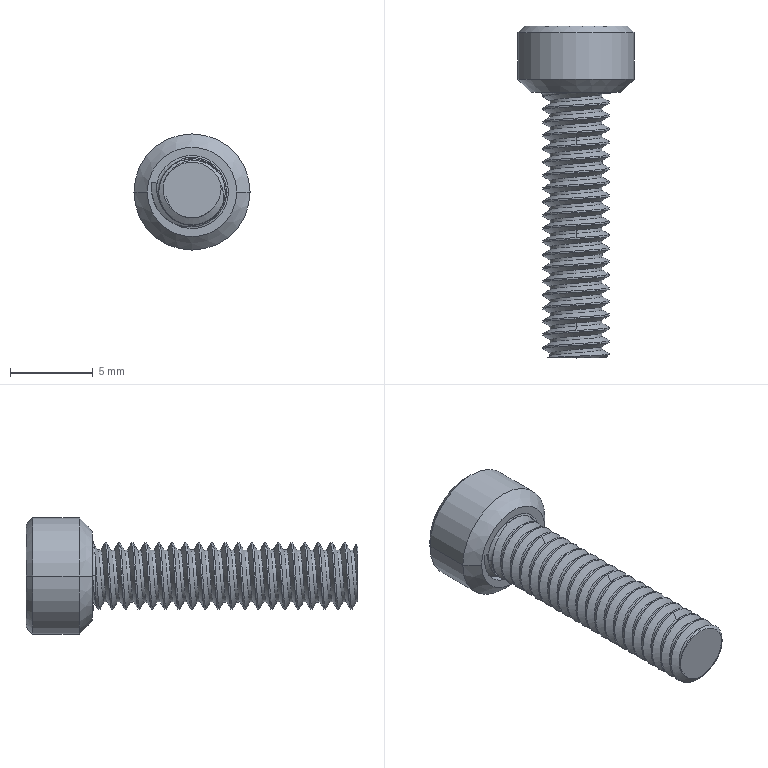Part | NX | features BREP 1 | 1 solid | 93 faces | box 7 x 20 x 7 mm | volume 283.89 mm3 | cylinder 45 | spline 21 | plane 16 | cone 8 | torus 3 | commonest cylinder face diameters 4 x41 4.173 x2 7 x2